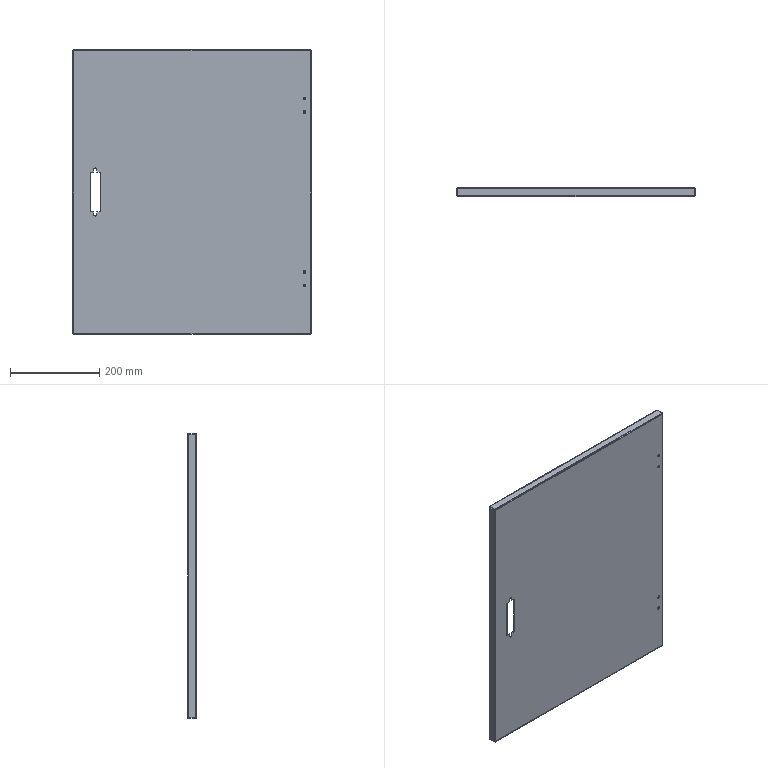Part | STEP file | JBJ-P-1011-09 | 1 solid | 90 faces | box 535 x 20 x 640 mm | volume 494626 mm3 | plane 48 | cylinder 26 | spline 16 | commonest cylinder face diameters 2 x8 4.4 x8 4 x4 6 x4 7 x2